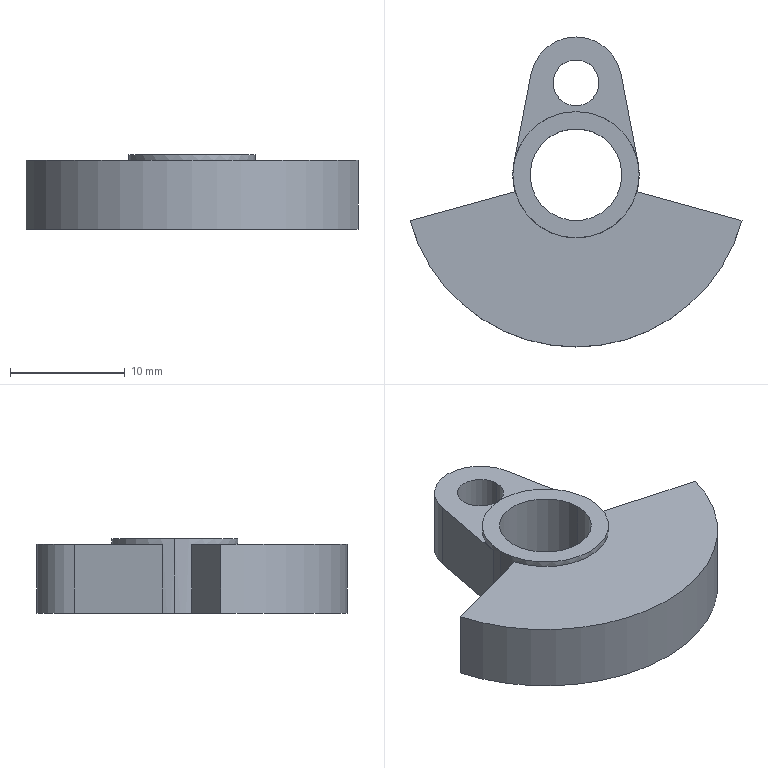Part | SolidWorks | features ICE 2, Extrusion 1 | 1 solid | 16 faces | box 28.914 x 27 x 6.5 mm | volume 2065 mm3 | cylinder 8 | plane 8 | commonest cylinder face diameters 8 x3 4 x2 11 x2 30 x1
STEP:
#1=CARTESIAN_POINT('',(-2.,8.,6.));
#2=VERTEX_POINT('',#1);
#3=CARTESIAN_POINT('',(2.,8.,6.));
#4=VERTEX_POINT('',#3);
#5=CARTESIAN_POINT('',(0.,8.,6.));
#6=DIRECTION('',(0.,0.,1.));
#7=DIRECTION('',(1.,0.,0.));
#8=AXIS2_PLACEMENT_3D('',#5,#6,#7);
#9=CIRCLE('',#8,2.);
#10=EDGE_CURVE('',#2,#4,#9,.T.);
#11=ORIENTED_EDGE('',*,*,#10,.T.);
#12=CARTESIAN_POINT('',(2.,8.,0.));
#13=VERTEX_POINT('',#12);
#14=CARTESIAN_POINT('',(2.,8.,6.));
#15=DIRECTION('',(0.,0.,-1.));
#16=VECTOR('',#15,1000.);
#17=LINE('',#14,#16);
#18=EDGE_CURVE('',#4,#13,#17,.T.);
#19=ORIENTED_EDGE('',*,*,#18,.T.);
#20=CARTESIAN_POINT('',(-2.,8.,0.));
#21=VERTEX_POINT('',#20);
#22=CARTESIAN_POINT('',(0.,8.,0.));
#23=DIRECTION('',(0.,0.,1.));
#24=DIRECTION('',(1.,0.,0.));
#25=AXIS2_PLACEMENT_3D('',#22,#23,#24);
#26=CIRCLE('',#25,2.);
#27=EDGE_CURVE('',#21,#13,#26,.T.);
#28=ORIENTED_EDGE('',*,*,#27,.F.);
#29=CARTESIAN_POINT('',(-2.,8.,6.));
#30=DIRECTION('',(0.,0.,-1.));
#31=VECTOR('',#30,1000.);
#32=LINE('',#29,#31);
#33=EDGE_CURVE('',#2,#21,#32,.T.);
#34=ORIENTED_EDGE('',*,*,#33,.F.);
#35=EDGE_LOOP('',(#11,#19,#28,#34));
#36=FACE_OUTER_BOUND('',#35,.T.);
#37=CARTESIAN_POINT('',(0.,8.,6.));
#38=DIRECTION('',(0.,0.,-1.));
#39=DIRECTION('',(-1.,0.,0.));
#40=AXIS2_PLACEMENT_3D('',#37,#38,#39);
#41=CYLINDRICAL_SURFACE('',#40,2.);
#42=ADVANCED_FACE('',(#36),#41,.F.);
#43=CARTESIAN_POINT('',(-4.,0.,6.5));
#44=VERTEX_POINT('',#43);
#45=CARTESIAN_POINT('',(4.,0.,6.5));
#46=VERTEX_POINT('',#45);
#47=CARTESIAN_POINT('',(0.,0.,6.5));
#48=DIRECTION('',(0.,0.,1.));
#49=DIRECTION('',(1.,0.,0.));
#50=AXIS2_PLACEMENT_3D('',#47,#48,#49);
#51=CIRCLE('',#50,4.);
#52=EDGE_CURVE('',#44,#46,#51,.T.);
#53=ORIENTED_EDGE('',*,*,#52,.T.);
#54=CARTESIAN_POINT('',(4.,0.,0.));
#55=VERTEX_POINT('',#54);
#56=CARTESIAN_POINT('',(4.,0.,6.));
#57=DIRECTION('',(0.,0.,-1.));
#58=VECTOR('',#57,1000.);
#59=LINE('',#56,#58);
#60=EDGE_CURVE('',#46,#55,#59,.T.);
#61=ORIENTED_EDGE('',*,*,#60,.T.);
#62=CARTESIAN_POINT('',(-4.,0.,0.));
#63=VERTEX_POINT('',#62);
#64=CARTESIAN_POINT('',(0.,0.,0.));
#65=DIRECTION('',(0.,0.,1.));
#66=DIRECTION('',(1.,0.,0.));
#67=AXIS2_PLACEMENT_3D('',#64,#65,#66);
#68=CIRCLE('',#67,4.);
#69=EDGE_CURVE('',#63,#55,#68,.T.);
#70=ORIENTED_EDGE('',*,*,#69,.F.);
#71=CARTESIAN_POINT('',(-4.,0.,6.));
#72=DIRECTION('',(0.,0.,-1.));
#73=VECTOR('',#72,1000.);
#74=LINE('',#71,#73);
#75=EDGE_CURVE('',#44,#63,#74,.T.);
#76=ORIENTED_EDGE('',*,*,#75,.F.);
#77=EDGE_LOOP('',(#53,#61,#70,#76));
#78=FACE_OUTER_BOUND('',#77,.T.);
#79=CARTESIAN_POINT('',(0.,0.,6.));
#80=DIRECTION('',(0.,0.,-1.));
#81=DIRECTION('',(-1.,0.,0.));
#82=AXIS2_PLACEMENT_3D('',#79,#80,#81);
#83=CYLINDRICAL_SURFACE('',#82,4.);
#84=ADVANCED_FACE('',(#78),#83,.F.);
#85=CARTESIAN_POINT('',(5.5,0.,6.5));
#86=VERTEX_POINT('',#85);
#87=CARTESIAN_POINT('',(-5.5,0.,6.5));
#88=VERTEX_POINT('',#87);
#89=CARTESIAN_POINT('',(0.,0.,6.5));
#90=DIRECTION('',(0.,0.,1.));
#91=DIRECTION('',(1.,0.,0.));
#92=AXIS2_PLACEMENT_3D('',#89,#90,#91);
#93=CIRCLE('',#92,5.5);
#94=EDGE_CURVE('',#86,#88,#93,.T.);
#95=ORIENTED_EDGE('',*,*,#94,.F.);
#96=CARTESIAN_POINT('',(5.5,0.,0.));
#97=VERTEX_POINT('',#96);
#98=CARTESIAN_POINT('',(5.5,0.,6.));
#99=DIRECTION('',(0.,0.,-1.));
#100=VECTOR('',#99,1000.);
#101=LINE('',#98,#100);
#102=EDGE_CURVE('',#86,#97,#101,.T.);
#103=ORIENTED_EDGE('',*,*,#102,.T.);
#104=CARTESIAN_POINT('',(5.402,1.031,0.));
#105=VERTEX_POINT('',#104);
#106=CARTESIAN_POINT('',(0.,0.,0.));
#107=DIRECTION('',(0.,0.,1.));
#108=DIRECTION('',(1.,0.,0.));
#109=AXIS2_PLACEMENT_3D('',#106,#107,#108);
#110=CIRCLE('',#109,5.5);
#111=EDGE_CURVE('',#97,#105,#110,.T.);
#112=ORIENTED_EDGE('',*,*,#111,.T.);
#113=CARTESIAN_POINT('',(5.402,1.031,6.));
#114=VERTEX_POINT('',#113);
#115=CARTESIAN_POINT('',(5.402,1.031,6.));
#116=DIRECTION('',(0.,0.,-1.));
#117=VECTOR('',#116,1000.);
#118=LINE('',#115,#117);
#119=EDGE_CURVE('',#114,#105,#118,.T.);
#120=ORIENTED_EDGE('',*,*,#119,.F.);
#121=CARTESIAN_POINT('',(-5.402,1.031,6.));
#122=VERTEX_POINT('',#121);
#123=CARTESIAN_POINT('',(0.,0.,6.));
#124=DIRECTION('',(0.,0.,1.));
#125=DIRECTION('',(1.,0.,0.));
#126=AXIS2_PLACEMENT_3D('',#123,#124,#125);
#127=CIRCLE('',#126,5.5);
#128=EDGE_CURVE('',#114,#122,#127,.T.);
#129=ORIENTED_EDGE('',*,*,#128,.T.);
#130=CARTESIAN_POINT('',(-5.402,1.031,0.));
#131=VERTEX_POINT('',#130);
#132=CARTESIAN_POINT('',(-5.402,1.031,6.));
#133=DIRECTION('',(0.,0.,-1.));
#134=VECTOR('',#133,1000.);
#135=LINE('',#132,#134);
#136=EDGE_CURVE('',#122,#131,#135,.T.);
#137=ORIENTED_EDGE('',*,*,#136,.T.);
#138=CARTESIAN_POINT('',(-5.5,0.,0.));
#139=VERTEX_POINT('',#138);
#140=CARTESIAN_POINT('',(0.,0.,0.));
#141=DIRECTION('',(0.,0.,1.));
#142=DIRECTION('',(1.,0.,0.));
#143=AXIS2_PLACEMENT_3D('',#140,#141,#142);
#144=CIRCLE('',#143,5.5);
#145=EDGE_CURVE('',#131,#139,#144,.T.);
#146=ORIENTED_EDGE('',*,*,#145,.T.);
#147=CARTESIAN_POINT('',(-5.5,0.,6.));
#148=DIRECTION('',(0.,0.,-1.));
#149=VECTOR('',#148,1000.);
#150=LINE('',#147,#149);
#151=EDGE_CURVE('',#88,#139,#150,.T.);
#152=ORIENTED_EDGE('',*,*,#151,.F.);
#153=EDGE_LOOP('',(#95,#103,#112,#120,#129,#137,#146,#152));
#154=FACE_OUTER_BOUND('',#153,.T.);
#155=CARTESIAN_POINT('',(0.,0.,6.));
#156=DIRECTION('',(0.,0.,-1.));
#157=DIRECTION('',(-1.,0.,0.));
#158=AXIS2_PLACEMENT_3D('',#155,#156,#157);
#159=CYLINDRICAL_SURFACE('',#158,5.5);
#160=ADVANCED_FACE('',(#154),#159,.T.);
#161=ORIENTED_EDGE('',*,*,#128,.F.);
#162=CARTESIAN_POINT('',(3.929,8.75,6.));
#163=VERTEX_POINT('',#162);
#164=CARTESIAN_POINT('',(3.929,8.75,6.));
#165=DIRECTION('',(-0.1875,0.9823,0.));
#166=VECTOR('',#165,1000.);
#167=LINE('',#164,#166);
#168=EDGE_CURVE('',#114,#163,#167,.T.);
#169=ORIENTED_EDGE('',*,*,#168,.T.);
#170=CARTESIAN_POINT('',(-3.929,8.75,6.));
#171=VERTEX_POINT('',#170);
#172=CARTESIAN_POINT('',(0.,8.,6.));
#173=DIRECTION('',(0.,0.,1.));
#174=DIRECTION('',(1.,0.,0.));
#175=AXIS2_PLACEMENT_3D('',#172,#173,#174);
#176=CIRCLE('',#175,4.);
#177=EDGE_CURVE('',#163,#171,#176,.T.);
#178=ORIENTED_EDGE('',*,*,#177,.T.);
#179=CARTESIAN_POINT('',(-3.929,8.75,6.));
#180=DIRECTION('',(-0.1875,-0.9823,0.));
#181=VECTOR('',#180,1000.);
#182=LINE('',#179,#181);
#183=EDGE_CURVE('',#171,#122,#182,.T.);
#184=ORIENTED_EDGE('',*,*,#183,.T.);
#185=EDGE_LOOP('',(#161,#169,#178,#184));
#186=FACE_OUTER_BOUND('',#185,.T.);
#187=ORIENTED_EDGE('',*,*,#10,.F.);
#188=CARTESIAN_POINT('',(0.,8.,6.));
#189=DIRECTION('',(0.,0.,1.));
#190=DIRECTION('',(1.,0.,0.));
#191=AXIS2_PLACEMENT_3D('',#188,#189,#190);
#192=CIRCLE('',#191,2.);
#193=EDGE_CURVE('',#4,#2,#192,.T.);
#194=ORIENTED_EDGE('',*,*,#193,.F.);
#195=EDGE_LOOP('',(#187,#194));
#196=FACE_BOUND('',#195,.T.);
#197=CARTESIAN_POINT('',(0.,0.,6.));
#198=DIRECTION('',(0.,0.,1.));
#199=DIRECTION('',(1.,0.,0.));
#200=AXIS2_PLACEMENT_3D('',#197,#198,#199);
#201=PLANE('',#200);
#202=ADVANCED_FACE('',(#186,#196),#201,.T.);
#203=CARTESIAN_POINT('',(-5.301,-1.467,6.));
#204=VERTEX_POINT('',#203);
#205=CARTESIAN_POINT('',(5.301,-1.467,6.));
#206=VERTEX_POINT('',#205);
#207=CARTESIAN_POINT('',(0.,0.,6.));
#208=DIRECTION('',(0.,0.,1.));
#209=DIRECTION('',(1.,0.,0.));
#210=AXIS2_PLACEMENT_3D('',#207,#208,#209);
#211=CIRCLE('',#210,5.5);
#212=EDGE_CURVE('',#204,#206,#211,.T.);
#213=ORIENTED_EDGE('',*,*,#212,.F.);
#214=CARTESIAN_POINT('',(-14.457,-4.,6.));
#215=VERTEX_POINT('',#214);
#216=CARTESIAN_POINT('',(-5.301,-1.467,6.));
#217=DIRECTION('',(-0.9638,-0.2667,0.));
#218=VECTOR('',#217,1000.);
#219=LINE('',#216,#218);
#220=EDGE_CURVE('',#204,#215,#219,.T.);
#221=ORIENTED_EDGE('',*,*,#220,.T.);
#222=CARTESIAN_POINT('',(14.457,-4.,6.));
#223=VERTEX_POINT('',#222);
#224=CARTESIAN_POINT('',(0.,0.,6.));
#225=DIRECTION('',(0.,0.,1.));
#226=DIRECTION('',(1.,0.,0.));
#227=AXIS2_PLACEMENT_3D('',#224,#225,#226);
#228=CIRCLE('',#227,15.);
#229=EDGE_CURVE('',#215,#223,#228,.T.);
#230=ORIENTED_EDGE('',*,*,#229,.T.);
#231=CARTESIAN_POINT('',(5.301,-1.467,6.));
#232=DIRECTION('',(-0.9638,0.2667,0.));
#233=VECTOR('',#232,1000.);
#234=LINE('',#231,#233);
#235=EDGE_CURVE('',#223,#206,#234,.T.);
#236=ORIENTED_EDGE('',*,*,#235,.T.);
#237=EDGE_LOOP('',(#213,#221,#230,#236));
#238=FACE_OUTER_BOUND('',#237,.T.);
#239=CARTESIAN_POINT('',(0.,0.,6.));
#240=DIRECTION('',(0.,0.,1.));
#241=DIRECTION('',(1.,0.,0.));
#242=AXIS2_PLACEMENT_3D('',#239,#240,#241);
#243=PLANE('',#242);
#244=ADVANCED_FACE('',(#238),#243,.T.);
#245=CARTESIAN_POINT('',(-14.457,-4.,0.));
#246=VERTEX_POINT('',#245);
#247=CARTESIAN_POINT('',(14.457,-4.,0.));
#248=VERTEX_POINT('',#247);
#249=CARTESIAN_POINT('',(0.,0.,0.));
#250=DIRECTION('',(0.,0.,1.));
#251=DIRECTION('',(1.,0.,0.));
#252=AXIS2_PLACEMENT_3D('',#249,#250,#251);
#253=CIRCLE('',#252,15.);
#254=EDGE_CURVE('',#246,#248,#253,.T.);
#255=ORIENTED_EDGE('',*,*,#254,.F.);
#256=CARTESIAN_POINT('',(-5.301,-1.467,0.));
#257=VERTEX_POINT('',#256);
#258=CARTESIAN_POINT('',(-5.301,-1.467,0.));
#259=DIRECTION('',(-0.9638,-0.2667,0.));
#260=VECTOR('',#259,1000.);
#261=LINE('',#258,#260);
#262=EDGE_CURVE('',#257,#246,#261,.T.);
#263=ORIENTED_EDGE('',*,*,#262,.F.);
#264=CARTESIAN_POINT('',(0.,0.,0.));
#265=DIRECTION('',(0.,0.,1.));
#266=DIRECTION('',(1.,0.,0.));
#267=AXIS2_PLACEMENT_3D('',#264,#265,#266);
#268=CIRCLE('',#267,5.5);
#269=EDGE_CURVE('',#139,#257,#268,.T.);
#270=ORIENTED_EDGE('',*,*,#269,.F.);
#271=ORIENTED_EDGE('',*,*,#145,.F.);
#272=CARTESIAN_POINT('',(-3.929,8.75,0.));
#273=VERTEX_POINT('',#272);
#274=CARTESIAN_POINT('',(-3.929,8.75,0.));
#275=DIRECTION('',(-0.1875,-0.9823,0.));
#276=VECTOR('',#275,1000.);
#277=LINE('',#274,#276);
#278=EDGE_CURVE('',#273,#131,#277,.T.);
#279=ORIENTED_EDGE('',*,*,#278,.F.);
#280=CARTESIAN_POINT('',(3.929,8.75,0.));
#281=VERTEX_POINT('',#280);
#282=CARTESIAN_POINT('',(0.,8.,0.));
#283=DIRECTION('',(0.,0.,1.));
#284=DIRECTION('',(1.,0.,0.));
#285=AXIS2_PLACEMENT_3D('',#282,#283,#284);
#286=CIRCLE('',#285,4.);
#287=EDGE_CURVE('',#281,#273,#286,.T.);
#288=ORIENTED_EDGE('',*,*,#287,.F.);
#289=CARTESIAN_POINT('',(3.929,8.75,0.));
#290=DIRECTION('',(-0.1875,0.9823,0.));
#291=VECTOR('',#290,1000.);
#292=LINE('',#289,#291);
#293=EDGE_CURVE('',#105,#281,#292,.T.);
#294=ORIENTED_EDGE('',*,*,#293,.F.);
#295=ORIENTED_EDGE('',*,*,#111,.F.);
#296=CARTESIAN_POINT('',(5.301,-1.467,0.));
#297=VERTEX_POINT('',#296);
#298=CARTESIAN_POINT('',(0.,0.,0.));
#299=DIRECTION('',(0.,0.,1.));
#300=DIRECTION('',(1.,0.,0.));
#301=AXIS2_PLACEMENT_3D('',#298,#299,#300);
#302=CIRCLE('',#301,5.5);
#303=EDGE_CURVE('',#297,#97,#302,.T.);
#304=ORIENTED_EDGE('',*,*,#303,.F.);
#305=CARTESIAN_POINT('',(5.301,-1.467,0.));
#306=DIRECTION('',(-0.9638,0.2667,0.));
#307=VECTOR('',#306,1000.);
#308=LINE('',#305,#307);
#309=EDGE_CURVE('',#248,#297,#308,.T.);
#310=ORIENTED_EDGE('',*,*,#309,.F.);
#311=EDGE_LOOP('',(#255,#263,#270,#271,#279,#288,#294,#295,#304,#310));
#312=FACE_OUTER_BOUND('',#311,.T.);
#313=ORIENTED_EDGE('',*,*,#69,.T.);
#314=CARTESIAN_POINT('',(0.,0.,0.));
#315=DIRECTION('',(0.,0.,1.));
#316=DIRECTION('',(1.,0.,0.));
#317=AXIS2_PLACEMENT_3D('',#314,#315,#316);
#318=CIRCLE('',#317,4.);
#319=EDGE_CURVE('',#55,#63,#318,.T.);
#320=ORIENTED_EDGE('',*,*,#319,.T.);
#321=EDGE_LOOP('',(#313,#320));
#322=FACE_BOUND('',#321,.T.);
#323=ORIENTED_EDGE('',*,*,#27,.T.);
#324=CARTESIAN_POINT('',(0.,8.,0.));
#325=DIRECTION('',(0.,0.,1.));
#326=DIRECTION('',(1.,0.,0.));
#327=AXIS2_PLACEMENT_3D('',#324,#325,#326);
#328=CIRCLE('',#327,2.);
#329=EDGE_CURVE('',#13,#21,#328,.T.);
#330=ORIENTED_EDGE('',*,*,#329,.T.);
#331=EDGE_LOOP('',(#323,#330));
#332=FACE_BOUND('',#331,.T.);
#333=CARTESIAN_POINT('',(0.,0.,0.));
#334=DIRECTION('',(0.,0.,1.));
#335=DIRECTION('',(1.,0.,0.));
#336=AXIS2_PLACEMENT_3D('',#333,#334,#335);
#337=PLANE('',#336);
#338=ADVANCED_FACE('',(#312,#322,#332),#337,.F.);
#339=ORIENTED_EDGE('',*,*,#254,.T.);
#340=CARTESIAN_POINT('',(14.457,-4.,6.));
#341=DIRECTION('',(0.,0.,-1.));
#342=VECTOR('',#341,1000.);
#343=LINE('',#340,#342);
#344=EDGE_CURVE('',#223,#248,#343,.T.);
#345=ORIENTED_EDGE('',*,*,#344,.F.);
#346=ORIENTED_EDGE('',*,*,#229,.F.);
#347=CARTESIAN_POINT('',(-14.457,-4.,6.));
#348=DIRECTION('',(0.,0.,-1.));
#349=VECTOR('',#348,1000.);
#350=LINE('',#347,#349);
#351=EDGE_CURVE('',#215,#246,#350,.T.);
#352=ORIENTED_EDGE('',*,*,#351,.T.);
#353=EDGE_LOOP('',(#339,#345,#346,#352));
#354=FACE_OUTER_BOUND('',#353,.T.);
#355=CARTESIAN_POINT('',(0.,0.,6.));
#356=DIRECTION('',(0.,0.,-1.));
#357=DIRECTION('',(-1.,0.,0.));
#358=AXIS2_PLACEMENT_3D('',#355,#356,#357);
#359=CYLINDRICAL_SURFACE('',#358,15.);
#360=ADVANCED_FACE('',(#354),#359,.T.);
#361=ORIENTED_EDGE('',*,*,#309,.T.);
#362=CARTESIAN_POINT('',(5.301,-1.467,6.));
#363=DIRECTION('',(0.,0.,-1.));
#364=VECTOR('',#363,1000.);
#365=LINE('',#362,#364);
#366=EDGE_CURVE('',#206,#297,#365,.T.);
#367=ORIENTED_EDGE('',*,*,#366,.F.);
#368=ORIENTED_EDGE('',*,*,#235,.F.);
#369=ORIENTED_EDGE('',*,*,#344,.T.);
#370=EDGE_LOOP('',(#361,#367,#368,#369));
#371=FACE_OUTER_BOUND('',#370,.T.);
#372=CARTESIAN_POINT('',(5.301,-1.467,6.));
#373=DIRECTION('',(-0.2667,-0.9638,0.));
#374=DIRECTION('',(0.9638,-0.2667,0.));
#375=AXIS2_PLACEMENT_3D('',#372,#373,#374);
#376=PLANE('',#375);
#377=ADVANCED_FACE('',(#371),#376,.F.);
#378=ORIENTED_EDGE('',*,*,#102,.F.);
#379=CARTESIAN_POINT('',(0.,0.,6.5));
#380=DIRECTION('',(0.,0.,1.));
#381=DIRECTION('',(1.,0.,0.));
#382=AXIS2_PLACEMENT_3D('',#379,#380,#381);
#383=CIRCLE('',#382,5.5);
#384=EDGE_CURVE('',#88,#86,#383,.T.);
#385=ORIENTED_EDGE('',*,*,#384,.F.);
#386=ORIENTED_EDGE('',*,*,#151,.T.);
#387=ORIENTED_EDGE('',*,*,#269,.T.);
#388=CARTESIAN_POINT('',(-5.301,-1.467,6.));
#389=DIRECTION('',(0.,0.,-1.));
#390=VECTOR('',#389,1000.);
#391=LINE('',#388,#390);
#392=EDGE_CURVE('',#204,#257,#391,.T.);
#393=ORIENTED_EDGE('',*,*,#392,.F.);
#394=ORIENTED_EDGE('',*,*,#212,.T.);
#395=ORIENTED_EDGE('',*,*,#366,.T.);
#396=ORIENTED_EDGE('',*,*,#303,.T.);
#397=EDGE_LOOP('',(#378,#385,#386,#387,#393,#394,#395,#396));
#398=FACE_OUTER_BOUND('',#397,.T.);
#399=CARTESIAN_POINT('',(0.,0.,6.));
#400=DIRECTION('',(0.,0.,-1.));
#401=DIRECTION('',(-1.,0.,0.));
#402=AXIS2_PLACEMENT_3D('',#399,#400,#401);
#403=CYLINDRICAL_SURFACE('',#402,5.5);
#404=ADVANCED_FACE('',(#398),#403,.T.);
#405=ORIENTED_EDGE('',*,*,#262,.T.);
#406=ORIENTED_EDGE('',*,*,#351,.F.);
#407=ORIENTED_EDGE('',*,*,#220,.F.);
#408=ORIENTED_EDGE('',*,*,#392,.T.);
#409=EDGE_LOOP('',(#405,#406,#407,#408));
#410=FACE_OUTER_BOUND('',#409,.T.);
#411=CARTESIAN_POINT('',(-5.301,-1.467,6.));
#412=DIRECTION('',(0.2667,-0.9638,0.));
#413=DIRECTION('',(0.9638,0.2667,0.));
#414=AXIS2_PLACEMENT_3D('',#411,#412,#413);
#415=PLANE('',#414);
#416=ADVANCED_FACE('',(#410),#415,.F.);
#417=ORIENTED_EDGE('',*,*,#60,.F.);
#418=CARTESIAN_POINT('',(0.,0.,6.5));
#419=DIRECTION('',(0.,0.,1.));
#420=DIRECTION('',(1.,0.,0.));
#421=AXIS2_PLACEMENT_3D('',#418,#419,#420);
#422=CIRCLE('',#421,4.);
#423=EDGE_CURVE('',#46,#44,#422,.T.);
#424=ORIENTED_EDGE('',*,*,#423,.T.);
#425=ORIENTED_EDGE('',*,*,#75,.T.);
#426=ORIENTED_EDGE('',*,*,#319,.F.);
#427=EDGE_LOOP('',(#417,#424,#425,#426));
#428=FACE_OUTER_BOUND('',#427,.T.);
#429=CARTESIAN_POINT('',(0.,0.,6.));
#430=DIRECTION('',(0.,0.,-1.));
#431=DIRECTION('',(-1.,0.,0.));
#432=AXIS2_PLACEMENT_3D('',#429,#430,#431);
#433=CYLINDRICAL_SURFACE('',#432,4.);
#434=ADVANCED_FACE('',(#428),#433,.F.);
#435=ORIENTED_EDGE('',*,*,#287,.T.);
#436=CARTESIAN_POINT('',(-3.929,8.75,6.));
#437=DIRECTION('',(0.,0.,-1.));
#438=VECTOR('',#437,1000.);
#439=LINE('',#436,#438);
#440=EDGE_CURVE('',#171,#273,#439,.T.);
#441=ORIENTED_EDGE('',*,*,#440,.F.);
#442=ORIENTED_EDGE('',*,*,#177,.F.);
#443=CARTESIAN_POINT('',(3.929,8.75,6.));
#444=DIRECTION('',(0.,0.,-1.));
#445=VECTOR('',#444,1000.);
#446=LINE('',#443,#445);
#447=EDGE_CURVE('',#163,#281,#446,.T.);
#448=ORIENTED_EDGE('',*,*,#447,.T.);
#449=EDGE_LOOP('',(#435,#441,#442,#448));
#450=FACE_OUTER_BOUND('',#449,.T.);
#451=CARTESIAN_POINT('',(0.,8.,6.));
#452=DIRECTION('',(0.,0.,-1.));
#453=DIRECTION('',(-1.,0.,0.));
#454=AXIS2_PLACEMENT_3D('',#451,#452,#453);
#455=CYLINDRICAL_SURFACE('',#454,4.);
#456=ADVANCED_FACE('',(#450),#455,.T.);
#457=ORIENTED_EDGE('',*,*,#278,.T.);
#458=ORIENTED_EDGE('',*,*,#136,.F.);
#459=ORIENTED_EDGE('',*,*,#183,.F.);
#460=ORIENTED_EDGE('',*,*,#440,.T.);
#461=EDGE_LOOP('',(#457,#458,#459,#460));
#462=FACE_OUTER_BOUND('',#461,.T.);
#463=CARTESIAN_POINT('',(-3.929,8.75,6.));
#464=DIRECTION('',(0.9823,-0.1875,0.));
#465=DIRECTION('',(0.1875,0.9823,0.));
#466=AXIS2_PLACEMENT_3D('',#463,#464,#465);
#467=PLANE('',#466);
#468=ADVANCED_FACE('',(#462),#467,.F.);
#469=ORIENTED_EDGE('',*,*,#293,.T.);
#470=ORIENTED_EDGE('',*,*,#447,.F.);
#471=ORIENTED_EDGE('',*,*,#168,.F.);
#472=ORIENTED_EDGE('',*,*,#119,.T.);
#473=EDGE_LOOP('',(#469,#470,#471,#472));
#474=FACE_OUTER_BOUND('',#473,.T.);
#475=CARTESIAN_POINT('',(3.929,8.75,6.));
#476=DIRECTION('',(-0.9823,-0.1875,0.));
#477=DIRECTION('',(0.1875,-0.9823,0.));
#478=AXIS2_PLACEMENT_3D('',#475,#476,#477);
#479=PLANE('',#478);
#480=ADVANCED_FACE('',(#474),#479,.F.);
#481=ORIENTED_EDGE('',*,*,#18,.F.);
#482=ORIENTED_EDGE('',*,*,#193,.T.);
#483=ORIENTED_EDGE('',*,*,#33,.T.);
#484=ORIENTED_EDGE('',*,*,#329,.F.);
#485=EDGE_LOOP('',(#481,#482,#483,#484));
#486=FACE_OUTER_BOUND('',#485,.T.);
#487=CARTESIAN_POINT('',(0.,8.,6.));
#488=DIRECTION('',(0.,0.,-1.));
#489=DIRECTION('',(-1.,0.,0.));
#490=AXIS2_PLACEMENT_3D('',#487,#488,#489);
#491=CYLINDRICAL_SURFACE('',#490,2.);
#492=ADVANCED_FACE('',(#486),#491,.F.);
#493=ORIENTED_EDGE('',*,*,#384,.T.);
#494=ORIENTED_EDGE('',*,*,#94,.T.);
#495=EDGE_LOOP('',(#493,#494));
#496=FACE_OUTER_BOUND('',#495,.T.);
#497=ORIENTED_EDGE('',*,*,#52,.F.);
#498=ORIENTED_EDGE('',*,*,#423,.F.);
#499=EDGE_LOOP('',(#497,#498));
#500=FACE_BOUND('',#499,.T.);
#501=CARTESIAN_POINT('',(0.,0.,6.5));
#502=DIRECTION('',(0.,0.,1.));
#503=DIRECTION('',(1.,0.,0.));
#504=AXIS2_PLACEMENT_3D('',#501,#502,#503);
#505=PLANE('',#504);
#506=ADVANCED_FACE('',(#496,#500),#505,.T.);
#507=CLOSED_SHELL('',(#42,#84,#160,#202,#244,#338,#360,#377,#404,#416,#434,#456,#468,#480,#492,#506));
#508=MANIFOLD_SOLID_BREP('',#507);
#509=CARTESIAN_POINT('',(0.,0.,0.));
#510=DIRECTION('',(0.,0.,1.));
#511=DIRECTION('',(1.,0.,0.));
#512=AXIS2_PLACEMENT_3D('',#509,#510,#511);
#513=(LENGTH_UNIT()NAMED_UNIT(*)SI_UNIT(.MILLI.,.METRE.));
#514=UNCERTAINTY_MEASURE_WITH_UNIT(LENGTH_MEASURE(0.00001),#513,'','');
#515=(NAMED_UNIT(*)PLANE_ANGLE_UNIT()SI_UNIT($,.RADIAN.));
#516=(NAMED_UNIT(*)SI_UNIT($,.STERADIAN.)SOLID_ANGLE_UNIT());
#517=(GEOMETRIC_REPRESENTATION_CONTEXT(3)GLOBAL_UNCERTAINTY_ASSIGNED_CONTEXT((#514))GLOBAL_UNIT_ASSIGNED_CONTEXT((#513,#515,#516))REPRESENTATION_CONTEXT('',''));
#518=ADVANCED_BREP_SHAPE_REPRESENTATION('',(#508,#512),#517);